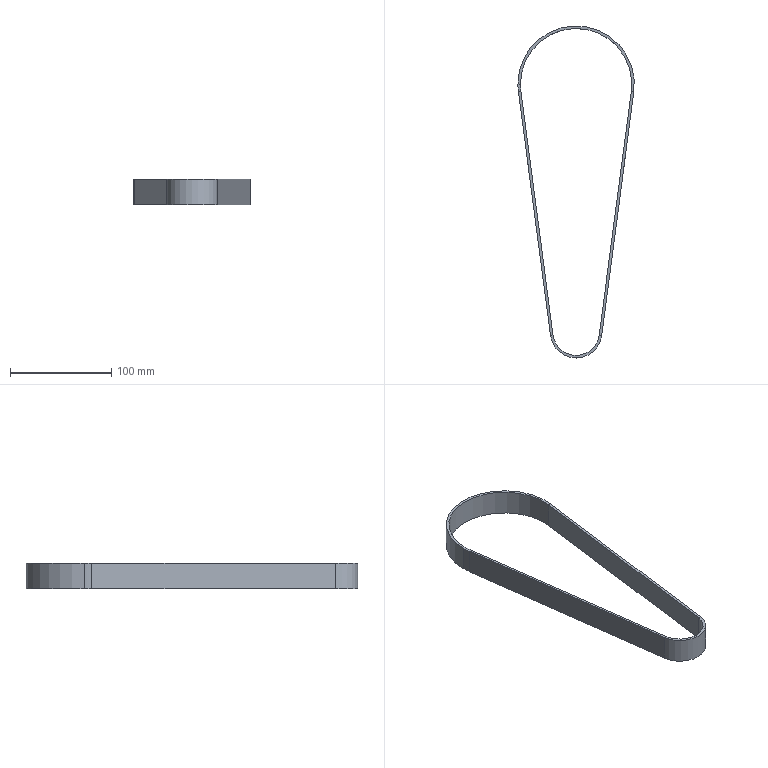Part | 1 solid | 20 faces | box 115 x 328 x 25 mm | volume 46693 mm3 | plane 14 | cylinder 6 | commonest cylinder face diameters 110 x2 115 x2 46 x1 51 x1
STEP:
#1=CARTESIAN_POINT('',(-54.529,-7.184,-12.5));
#2=VERTEX_POINT('',#1);
#3=CARTESIAN_POINT('',(-55.,0.,-12.5));
#4=VERTEX_POINT('',#3);
#5=CARTESIAN_POINT('',(0.,0.,-12.5));
#6=DIRECTION('',(0.,0.,-1.));
#7=DIRECTION('',(-0.9914,-0.1306,0.));
#8=AXIS2_PLACEMENT_3D('',#5,#6,#7);
#9=CIRCLE('',#8,55.);
#10=EDGE_CURVE('',#2,#4,#9,.T.);
#11=ORIENTED_EDGE('',*,*,#10,.F.);
#12=CARTESIAN_POINT('',(-57.007,-7.51,-12.5));
#13=VERTEX_POINT('',#12);
#14=CARTESIAN_POINT('',(-57.007,-7.51,-12.5));
#15=DIRECTION('',(-0.9914,-0.1306,0.));
#16=VECTOR('',#15,1000.);
#17=LINE('',#14,#16);
#18=EDGE_CURVE('',#2,#13,#17,.T.);
#19=ORIENTED_EDGE('',*,*,#18,.T.);
#20=CARTESIAN_POINT('',(-57.5,0.,-12.5));
#21=VERTEX_POINT('',#20);
#22=CARTESIAN_POINT('',(0.,0.,-12.5));
#23=DIRECTION('',(0.,0.,-1.));
#24=DIRECTION('',(-0.9914,-0.1306,0.));
#25=AXIS2_PLACEMENT_3D('',#22,#23,#24);
#26=CIRCLE('',#25,57.5);
#27=EDGE_CURVE('',#13,#21,#26,.T.);
#28=ORIENTED_EDGE('',*,*,#27,.T.);
#29=CARTESIAN_POINT('',(-57.5,0.,-12.5));
#30=DIRECTION('',(-1.,0.,0.));
#31=VECTOR('',#30,1000.);
#32=LINE('',#29,#31);
#33=EDGE_CURVE('',#4,#21,#32,.T.);
#34=ORIENTED_EDGE('',*,*,#33,.F.);
#35=EDGE_LOOP('',(#11,#19,#28,#34));
#36=FACE_OUTER_BOUND('',#35,.T.);
#37=CARTESIAN_POINT('',(-57.007,-7.51,-12.5));
#38=DIRECTION('',(0.,0.,-1.));
#39=DIRECTION('',(-1.,0.,0.));
#40=AXIS2_PLACEMENT_3D('',#37,#38,#39);
#41=PLANE('',#40);
#42=ADVANCED_FACE('',(#36),#41,.T.);
#43=CARTESIAN_POINT('',(-54.529,-7.184,12.5));
#44=VERTEX_POINT('',#43);
#45=CARTESIAN_POINT('',(-55.,0.,12.5));
#46=VERTEX_POINT('',#45);
#47=CARTESIAN_POINT('',(0.,0.,12.5));
#48=DIRECTION('',(0.,0.,-1.));
#49=DIRECTION('',(-0.9914,-0.1306,0.));
#50=AXIS2_PLACEMENT_3D('',#47,#48,#49);
#51=CIRCLE('',#50,55.);
#52=EDGE_CURVE('',#44,#46,#51,.T.);
#53=ORIENTED_EDGE('',*,*,#52,.F.);
#54=CARTESIAN_POINT('',(-54.529,-7.184,-12.5));
#55=DIRECTION('',(0.,0.,-1.));
#56=VECTOR('',#55,1000.);
#57=LINE('',#54,#56);
#58=EDGE_CURVE('',#44,#2,#57,.T.);
#59=ORIENTED_EDGE('',*,*,#58,.T.);
#60=ORIENTED_EDGE('',*,*,#10,.T.);
#61=CARTESIAN_POINT('',(-55.,0.,-12.5));
#62=DIRECTION('',(0.,0.,-1.));
#63=VECTOR('',#62,1000.);
#64=LINE('',#61,#63);
#65=EDGE_CURVE('',#46,#4,#64,.T.);
#66=ORIENTED_EDGE('',*,*,#65,.F.);
#67=EDGE_LOOP('',(#53,#59,#60,#66));
#68=FACE_OUTER_BOUND('',#67,.T.);
#69=CARTESIAN_POINT('',(0.,0.,0.));
#70=DIRECTION('',(0.,0.,-1.));
#71=DIRECTION('',(-1.,0.,0.));
#72=AXIS2_PLACEMENT_3D('',#69,#70,#71);
#73=CYLINDRICAL_SURFACE('',#72,55.);
#74=ADVANCED_FACE('',(#68),#73,.F.);
#75=CARTESIAN_POINT('',(-57.007,-7.51,12.5));
#76=VERTEX_POINT('',#75);
#77=CARTESIAN_POINT('',(-57.5,0.,12.5));
#78=VERTEX_POINT('',#77);
#79=CARTESIAN_POINT('',(0.,0.,12.5));
#80=DIRECTION('',(0.,0.,-1.));
#81=DIRECTION('',(-0.9914,-0.1306,0.));
#82=AXIS2_PLACEMENT_3D('',#79,#80,#81);
#83=CIRCLE('',#82,57.5);
#84=EDGE_CURVE('',#76,#78,#83,.T.);
#85=ORIENTED_EDGE('',*,*,#84,.F.);
#86=CARTESIAN_POINT('',(-57.007,-7.51,12.5));
#87=DIRECTION('',(0.9914,0.1306,0.));
#88=VECTOR('',#87,1000.);
#89=LINE('',#86,#88);
#90=EDGE_CURVE('',#76,#44,#89,.T.);
#91=ORIENTED_EDGE('',*,*,#90,.T.);
#92=ORIENTED_EDGE('',*,*,#52,.T.);
#93=CARTESIAN_POINT('',(-57.5,0.,12.5));
#94=DIRECTION('',(1.,0.,0.));
#95=VECTOR('',#94,1000.);
#96=LINE('',#93,#95);
#97=EDGE_CURVE('',#78,#46,#96,.T.);
#98=ORIENTED_EDGE('',*,*,#97,.F.);
#99=EDGE_LOOP('',(#85,#91,#92,#98));
#100=FACE_OUTER_BOUND('',#99,.T.);
#101=CARTESIAN_POINT('',(-57.007,-7.51,12.5));
#102=DIRECTION('',(0.,0.,1.));
#103=DIRECTION('',(1.,0.,0.));
#104=AXIS2_PLACEMENT_3D('',#101,#102,#103);
#105=PLANE('',#104);
#106=ADVANCED_FACE('',(#100),#105,.T.);
#107=ORIENTED_EDGE('',*,*,#18,.F.);
#108=CARTESIAN_POINT('',(-22.803,-248.004,-12.5));
#109=VERTEX_POINT('',#108);
#110=CARTESIAN_POINT('',(-22.803,-248.004,-12.5));
#111=DIRECTION('',(-0.1306,0.9914,0.));
#112=VECTOR('',#111,1000.);
#113=LINE('',#110,#112);
#114=EDGE_CURVE('',#109,#2,#113,.T.);
#115=ORIENTED_EDGE('',*,*,#114,.F.);
#116=CARTESIAN_POINT('',(-25.282,-248.331,-12.5));
#117=VERTEX_POINT('',#116);
#118=CARTESIAN_POINT('',(-25.282,-248.331,-12.5));
#119=DIRECTION('',(-0.9914,-0.1306,0.));
#120=VECTOR('',#119,1000.);
#121=LINE('',#118,#120);
#122=EDGE_CURVE('',#109,#117,#121,.T.);
#123=ORIENTED_EDGE('',*,*,#122,.T.);
#124=CARTESIAN_POINT('',(-25.282,-248.331,-12.5));
#125=DIRECTION('',(-0.1306,0.9914,0.));
#126=VECTOR('',#125,1000.);
#127=LINE('',#124,#126);
#128=EDGE_CURVE('',#117,#13,#127,.T.);
#129=ORIENTED_EDGE('',*,*,#128,.T.);
#130=EDGE_LOOP('',(#107,#115,#123,#129));
#131=FACE_OUTER_BOUND('',#130,.T.);
#132=CARTESIAN_POINT('',(-25.282,-248.331,-12.5));
#133=DIRECTION('',(0.,0.,-1.));
#134=DIRECTION('',(-1.,0.,0.));
#135=AXIS2_PLACEMENT_3D('',#132,#133,#134);
#136=PLANE('',#135);
#137=ADVANCED_FACE('',(#131),#136,.T.);
#138=ORIENTED_EDGE('',*,*,#114,.T.);
#139=ORIENTED_EDGE('',*,*,#58,.F.);
#140=CARTESIAN_POINT('',(-22.803,-248.004,12.5));
#141=VERTEX_POINT('',#140);
#142=CARTESIAN_POINT('',(-22.803,-248.004,12.5));
#143=DIRECTION('',(-0.1306,0.9914,0.));
#144=VECTOR('',#143,1000.);
#145=LINE('',#142,#144);
#146=EDGE_CURVE('',#141,#44,#145,.T.);
#147=ORIENTED_EDGE('',*,*,#146,.F.);
#148=CARTESIAN_POINT('',(-22.803,-248.004,-12.5));
#149=DIRECTION('',(0.,0.,-1.));
#150=VECTOR('',#149,1000.);
#151=LINE('',#148,#150);
#152=EDGE_CURVE('',#141,#109,#151,.T.);
#153=ORIENTED_EDGE('',*,*,#152,.T.);
#154=EDGE_LOOP('',(#138,#139,#147,#153));
#155=FACE_OUTER_BOUND('',#154,.T.);
#156=CARTESIAN_POINT('',(-22.803,-248.004,-12.5));
#157=DIRECTION('',(0.9914,0.1306,0.));
#158=DIRECTION('',(-0.1306,0.9914,0.));
#159=AXIS2_PLACEMENT_3D('',#156,#157,#158);
#160=PLANE('',#159);
#161=ADVANCED_FACE('',(#155),#160,.T.);
#162=ORIENTED_EDGE('',*,*,#146,.T.);
#163=ORIENTED_EDGE('',*,*,#90,.F.);
#164=CARTESIAN_POINT('',(-25.282,-248.331,12.5));
#165=VERTEX_POINT('',#164);
#166=CARTESIAN_POINT('',(-25.282,-248.331,12.5));
#167=DIRECTION('',(-0.1306,0.9914,0.));
#168=VECTOR('',#167,1000.);
#169=LINE('',#166,#168);
#170=EDGE_CURVE('',#165,#76,#169,.T.);
#171=ORIENTED_EDGE('',*,*,#170,.F.);
#172=CARTESIAN_POINT('',(-25.282,-248.331,12.5));
#173=DIRECTION('',(0.9914,0.1306,0.));
#174=VECTOR('',#173,1000.);
#175=LINE('',#172,#174);
#176=EDGE_CURVE('',#165,#141,#175,.T.);
#177=ORIENTED_EDGE('',*,*,#176,.T.);
#178=EDGE_LOOP('',(#162,#163,#171,#177));
#179=FACE_OUTER_BOUND('',#178,.T.);
#180=CARTESIAN_POINT('',(-25.282,-248.331,12.5));
#181=DIRECTION('',(0.,0.,1.));
#182=DIRECTION('',(1.,0.,0.));
#183=AXIS2_PLACEMENT_3D('',#180,#181,#182);
#184=PLANE('',#183);
#185=ADVANCED_FACE('',(#179),#184,.T.);
#186=ORIENTED_EDGE('',*,*,#170,.T.);
#187=CARTESIAN_POINT('',(-57.007,-7.51,-12.5));
#188=DIRECTION('',(0.,0.,1.));
#189=VECTOR('',#188,1000.);
#190=LINE('',#187,#189);
#191=EDGE_CURVE('',#13,#76,#190,.T.);
#192=ORIENTED_EDGE('',*,*,#191,.F.);
#193=ORIENTED_EDGE('',*,*,#128,.F.);
#194=CARTESIAN_POINT('',(-25.282,-248.331,-12.5));
#195=DIRECTION('',(0.,0.,1.));
#196=VECTOR('',#195,1000.);
#197=LINE('',#194,#196);
#198=EDGE_CURVE('',#117,#165,#197,.T.);
#199=ORIENTED_EDGE('',*,*,#198,.T.);
#200=EDGE_LOOP('',(#186,#192,#193,#199));
#201=FACE_OUTER_BOUND('',#200,.T.);
#202=CARTESIAN_POINT('',(-25.282,-248.331,-12.5));
#203=DIRECTION('',(-0.9914,-0.1306,0.));
#204=DIRECTION('',(0.1306,-0.9914,0.));
#205=AXIS2_PLACEMENT_3D('',#202,#203,#204);
#206=PLANE('',#205);
#207=ADVANCED_FACE('',(#201),#206,.T.);
#208=ORIENTED_EDGE('',*,*,#122,.F.);
#209=CARTESIAN_POINT('',(22.803,-248.004,-12.5));
#210=VERTEX_POINT('',#209);
#211=CARTESIAN_POINT('',(0.,-245.,-12.5));
#212=DIRECTION('',(0.,0.,-1.));
#213=DIRECTION('',(0.9914,-0.1306,0.));
#214=AXIS2_PLACEMENT_3D('',#211,#212,#213);
#215=CIRCLE('',#214,23.);
#216=EDGE_CURVE('',#210,#109,#215,.T.);
#217=ORIENTED_EDGE('',*,*,#216,.F.);
#218=CARTESIAN_POINT('',(25.282,-248.331,-12.5));
#219=VERTEX_POINT('',#218);
#220=CARTESIAN_POINT('',(25.282,-248.331,-12.5));
#221=DIRECTION('',(0.9914,-0.1306,0.));
#222=VECTOR('',#221,1000.);
#223=LINE('',#220,#222);
#224=EDGE_CURVE('',#210,#219,#223,.T.);
#225=ORIENTED_EDGE('',*,*,#224,.T.);
#226=CARTESIAN_POINT('',(0.,-245.,-12.5));
#227=DIRECTION('',(0.,0.,-1.));
#228=DIRECTION('',(0.9914,-0.1306,0.));
#229=AXIS2_PLACEMENT_3D('',#226,#227,#228);
#230=CIRCLE('',#229,25.5);
#231=EDGE_CURVE('',#219,#117,#230,.T.);
#232=ORIENTED_EDGE('',*,*,#231,.T.);
#233=EDGE_LOOP('',(#208,#217,#225,#232));
#234=FACE_OUTER_BOUND('',#233,.T.);
#235=CARTESIAN_POINT('',(25.282,-248.331,-12.5));
#236=DIRECTION('',(0.,0.,-1.));
#237=DIRECTION('',(-1.,0.,0.));
#238=AXIS2_PLACEMENT_3D('',#235,#236,#237);
#239=PLANE('',#238);
#240=ADVANCED_FACE('',(#234),#239,.T.);
#241=ORIENTED_EDGE('',*,*,#216,.T.);
#242=ORIENTED_EDGE('',*,*,#152,.F.);
#243=CARTESIAN_POINT('',(22.803,-248.004,12.5));
#244=VERTEX_POINT('',#243);
#245=CARTESIAN_POINT('',(0.,-245.,12.5));
#246=DIRECTION('',(0.,0.,-1.));
#247=DIRECTION('',(0.9914,-0.1306,0.));
#248=AXIS2_PLACEMENT_3D('',#245,#246,#247);
#249=CIRCLE('',#248,23.);
#250=EDGE_CURVE('',#244,#141,#249,.T.);
#251=ORIENTED_EDGE('',*,*,#250,.F.);
#252=CARTESIAN_POINT('',(22.803,-248.004,-12.5));
#253=DIRECTION('',(0.,0.,-1.));
#254=VECTOR('',#253,1000.);
#255=LINE('',#252,#254);
#256=EDGE_CURVE('',#244,#210,#255,.T.);
#257=ORIENTED_EDGE('',*,*,#256,.T.);
#258=EDGE_LOOP('',(#241,#242,#251,#257));
#259=FACE_OUTER_BOUND('',#258,.T.);
#260=CARTESIAN_POINT('',(0.,-245.,0.));
#261=DIRECTION('',(0.,0.,-1.));
#262=DIRECTION('',(-1.,0.,0.));
#263=AXIS2_PLACEMENT_3D('',#260,#261,#262);
#264=CYLINDRICAL_SURFACE('',#263,23.);
#265=ADVANCED_FACE('',(#259),#264,.F.);
#266=ORIENTED_EDGE('',*,*,#250,.T.);
#267=ORIENTED_EDGE('',*,*,#176,.F.);
#268=CARTESIAN_POINT('',(25.282,-248.331,12.5));
#269=VERTEX_POINT('',#268);
#270=CARTESIAN_POINT('',(0.,-245.,12.5));
#271=DIRECTION('',(0.,0.,-1.));
#272=DIRECTION('',(0.9914,-0.1306,0.));
#273=AXIS2_PLACEMENT_3D('',#270,#271,#272);
#274=CIRCLE('',#273,25.5);
#275=EDGE_CURVE('',#269,#165,#274,.T.);
#276=ORIENTED_EDGE('',*,*,#275,.F.);
#277=CARTESIAN_POINT('',(25.282,-248.331,12.5));
#278=DIRECTION('',(-0.9914,0.1306,0.));
#279=VECTOR('',#278,1000.);
#280=LINE('',#277,#279);
#281=EDGE_CURVE('',#269,#244,#280,.T.);
#282=ORIENTED_EDGE('',*,*,#281,.T.);
#283=EDGE_LOOP('',(#266,#267,#276,#282));
#284=FACE_OUTER_BOUND('',#283,.T.);
#285=CARTESIAN_POINT('',(25.282,-248.331,12.5));
#286=DIRECTION('',(0.,0.,1.));
#287=DIRECTION('',(1.,0.,0.));
#288=AXIS2_PLACEMENT_3D('',#285,#286,#287);
#289=PLANE('',#288);
#290=ADVANCED_FACE('',(#284),#289,.T.);
#291=ORIENTED_EDGE('',*,*,#275,.T.);
#292=ORIENTED_EDGE('',*,*,#198,.F.);
#293=ORIENTED_EDGE('',*,*,#231,.F.);
#294=CARTESIAN_POINT('',(25.282,-248.331,-12.5));
#295=DIRECTION('',(0.,0.,1.));
#296=VECTOR('',#295,1000.);
#297=LINE('',#294,#296);
#298=EDGE_CURVE('',#219,#269,#297,.T.);
#299=ORIENTED_EDGE('',*,*,#298,.T.);
#300=EDGE_LOOP('',(#291,#292,#293,#299));
#301=FACE_OUTER_BOUND('',#300,.T.);
#302=CARTESIAN_POINT('',(0.,-245.,0.));
#303=DIRECTION('',(0.,0.,-1.));
#304=DIRECTION('',(-1.,0.,0.));
#305=AXIS2_PLACEMENT_3D('',#302,#303,#304);
#306=CYLINDRICAL_SURFACE('',#305,25.5);
#307=ADVANCED_FACE('',(#301),#306,.T.);
#308=ORIENTED_EDGE('',*,*,#224,.F.);
#309=CARTESIAN_POINT('',(54.529,-7.184,-12.5));
#310=VERTEX_POINT('',#309);
#311=CARTESIAN_POINT('',(54.529,-7.184,-12.5));
#312=DIRECTION('',(-0.1306,-0.9914,0.));
#313=VECTOR('',#312,1000.);
#314=LINE('',#311,#313);
#315=EDGE_CURVE('',#310,#210,#314,.T.);
#316=ORIENTED_EDGE('',*,*,#315,.F.);
#317=CARTESIAN_POINT('',(57.007,-7.51,-12.5));
#318=VERTEX_POINT('',#317);
#319=CARTESIAN_POINT('',(57.007,-7.51,-12.5));
#320=DIRECTION('',(0.9914,-0.1306,0.));
#321=VECTOR('',#320,1000.);
#322=LINE('',#319,#321);
#323=EDGE_CURVE('',#310,#318,#322,.T.);
#324=ORIENTED_EDGE('',*,*,#323,.T.);
#325=CARTESIAN_POINT('',(57.007,-7.51,-12.5));
#326=DIRECTION('',(-0.1306,-0.9914,0.));
#327=VECTOR('',#326,1000.);
#328=LINE('',#325,#327);
#329=EDGE_CURVE('',#318,#219,#328,.T.);
#330=ORIENTED_EDGE('',*,*,#329,.T.);
#331=EDGE_LOOP('',(#308,#316,#324,#330));
#332=FACE_OUTER_BOUND('',#331,.T.);
#333=CARTESIAN_POINT('',(57.007,-7.51,-12.5));
#334=DIRECTION('',(0.,0.,-1.));
#335=DIRECTION('',(-1.,0.,0.));
#336=AXIS2_PLACEMENT_3D('',#333,#334,#335);
#337=PLANE('',#336);
#338=ADVANCED_FACE('',(#332),#337,.T.);
#339=ORIENTED_EDGE('',*,*,#315,.T.);
#340=ORIENTED_EDGE('',*,*,#256,.F.);
#341=CARTESIAN_POINT('',(54.529,-7.184,12.5));
#342=VERTEX_POINT('',#341);
#343=CARTESIAN_POINT('',(54.529,-7.184,12.5));
#344=DIRECTION('',(-0.1306,-0.9914,0.));
#345=VECTOR('',#344,1000.);
#346=LINE('',#343,#345);
#347=EDGE_CURVE('',#342,#244,#346,.T.);
#348=ORIENTED_EDGE('',*,*,#347,.F.);
#349=CARTESIAN_POINT('',(54.529,-7.184,-12.5));
#350=DIRECTION('',(0.,0.,-1.));
#351=VECTOR('',#350,1000.);
#352=LINE('',#349,#351);
#353=EDGE_CURVE('',#342,#310,#352,.T.);
#354=ORIENTED_EDGE('',*,*,#353,.T.);
#355=EDGE_LOOP('',(#339,#340,#348,#354));
#356=FACE_OUTER_BOUND('',#355,.T.);
#357=CARTESIAN_POINT('',(54.529,-7.184,-12.5));
#358=DIRECTION('',(-0.9914,0.1306,0.));
#359=DIRECTION('',(-0.1306,-0.9914,0.));
#360=AXIS2_PLACEMENT_3D('',#357,#358,#359);
#361=PLANE('',#360);
#362=ADVANCED_FACE('',(#356),#361,.T.);
#363=ORIENTED_EDGE('',*,*,#347,.T.);
#364=ORIENTED_EDGE('',*,*,#281,.F.);
#365=CARTESIAN_POINT('',(57.007,-7.51,12.5));
#366=VERTEX_POINT('',#365);
#367=CARTESIAN_POINT('',(57.007,-7.51,12.5));
#368=DIRECTION('',(-0.1306,-0.9914,0.));
#369=VECTOR('',#368,1000.);
#370=LINE('',#367,#369);
#371=EDGE_CURVE('',#366,#269,#370,.T.);
#372=ORIENTED_EDGE('',*,*,#371,.F.);
#373=CARTESIAN_POINT('',(57.007,-7.51,12.5));
#374=DIRECTION('',(-0.9914,0.1306,0.));
#375=VECTOR('',#374,1000.);
#376=LINE('',#373,#375);
#377=EDGE_CURVE('',#366,#342,#376,.T.);
#378=ORIENTED_EDGE('',*,*,#377,.T.);
#379=EDGE_LOOP('',(#363,#364,#372,#378));
#380=FACE_OUTER_BOUND('',#379,.T.);
#381=CARTESIAN_POINT('',(57.007,-7.51,12.5));
#382=DIRECTION('',(0.,0.,1.));
#383=DIRECTION('',(1.,0.,0.));
#384=AXIS2_PLACEMENT_3D('',#381,#382,#383);
#385=PLANE('',#384);
#386=ADVANCED_FACE('',(#380),#385,.T.);
#387=ORIENTED_EDGE('',*,*,#371,.T.);
#388=ORIENTED_EDGE('',*,*,#298,.F.);
#389=ORIENTED_EDGE('',*,*,#329,.F.);
#390=CARTESIAN_POINT('',(57.007,-7.51,-12.5));
#391=DIRECTION('',(0.,0.,1.));
#392=VECTOR('',#391,1000.);
#393=LINE('',#390,#392);
#394=EDGE_CURVE('',#318,#366,#393,.T.);
#395=ORIENTED_EDGE('',*,*,#394,.T.);
#396=EDGE_LOOP('',(#387,#388,#389,#395));
#397=FACE_OUTER_BOUND('',#396,.T.);
#398=CARTESIAN_POINT('',(57.007,-7.51,-12.5));
#399=DIRECTION('',(0.9914,-0.1306,0.));
#400=DIRECTION('',(0.1306,0.9914,0.));
#401=AXIS2_PLACEMENT_3D('',#398,#399,#400);
#402=PLANE('',#401);
#403=ADVANCED_FACE('',(#397),#402,.T.);
#404=ORIENTED_EDGE('',*,*,#323,.F.);
#405=CARTESIAN_POINT('',(0.,0.,-12.5));
#406=DIRECTION('',(0.,0.,-1.));
#407=DIRECTION('',(-1.,0.,0.));
#408=AXIS2_PLACEMENT_3D('',#405,#406,#407);
#409=CIRCLE('',#408,55.);
#410=EDGE_CURVE('',#4,#310,#409,.T.);
#411=ORIENTED_EDGE('',*,*,#410,.F.);
#412=ORIENTED_EDGE('',*,*,#33,.T.);
#413=CARTESIAN_POINT('',(0.,0.,-12.5));
#414=DIRECTION('',(0.,0.,-1.));
#415=DIRECTION('',(-1.,0.,0.));
#416=AXIS2_PLACEMENT_3D('',#413,#414,#415);
#417=CIRCLE('',#416,57.5);
#418=EDGE_CURVE('',#21,#318,#417,.T.);
#419=ORIENTED_EDGE('',*,*,#418,.T.);
#420=EDGE_LOOP('',(#404,#411,#412,#419));
#421=FACE_OUTER_BOUND('',#420,.T.);
#422=CARTESIAN_POINT('',(-57.5,0.,-12.5));
#423=DIRECTION('',(0.,0.,-1.));
#424=DIRECTION('',(-1.,0.,0.));
#425=AXIS2_PLACEMENT_3D('',#422,#423,#424);
#426=PLANE('',#425);
#427=ADVANCED_FACE('',(#421),#426,.T.);
#428=ORIENTED_EDGE('',*,*,#410,.T.);
#429=ORIENTED_EDGE('',*,*,#353,.F.);
#430=CARTESIAN_POINT('',(0.,0.,12.5));
#431=DIRECTION('',(0.,0.,-1.));
#432=DIRECTION('',(-1.,0.,0.));
#433=AXIS2_PLACEMENT_3D('',#430,#431,#432);
#434=CIRCLE('',#433,55.);
#435=EDGE_CURVE('',#46,#342,#434,.T.);
#436=ORIENTED_EDGE('',*,*,#435,.F.);
#437=ORIENTED_EDGE('',*,*,#65,.T.);
#438=EDGE_LOOP('',(#428,#429,#436,#437));
#439=FACE_OUTER_BOUND('',#438,.T.);
#440=CARTESIAN_POINT('',(0.,0.,0.));
#441=DIRECTION('',(0.,0.,-1.));
#442=DIRECTION('',(-1.,0.,0.));
#443=AXIS2_PLACEMENT_3D('',#440,#441,#442);
#444=CYLINDRICAL_SURFACE('',#443,55.);
#445=ADVANCED_FACE('',(#439),#444,.F.);
#446=ORIENTED_EDGE('',*,*,#435,.T.);
#447=ORIENTED_EDGE('',*,*,#377,.F.);
#448=CARTESIAN_POINT('',(0.,0.,12.5));
#449=DIRECTION('',(0.,0.,-1.));
#450=DIRECTION('',(-1.,0.,0.));
#451=AXIS2_PLACEMENT_3D('',#448,#449,#450);
#452=CIRCLE('',#451,57.5);
#453=EDGE_CURVE('',#78,#366,#452,.T.);
#454=ORIENTED_EDGE('',*,*,#453,.F.);
#455=ORIENTED_EDGE('',*,*,#97,.T.);
#456=EDGE_LOOP('',(#446,#447,#454,#455));
#457=FACE_OUTER_BOUND('',#456,.T.);
#458=CARTESIAN_POINT('',(-57.5,0.,12.5));
#459=DIRECTION('',(0.,0.,1.));
#460=DIRECTION('',(1.,0.,0.));
#461=AXIS2_PLACEMENT_3D('',#458,#459,#460);
#462=PLANE('',#461);
#463=ADVANCED_FACE('',(#457),#462,.T.);
#464=ORIENTED_EDGE('',*,*,#453,.T.);
#465=ORIENTED_EDGE('',*,*,#394,.F.);
#466=ORIENTED_EDGE('',*,*,#418,.F.);
#467=CARTESIAN_POINT('',(-57.5,0.,-12.5));
#468=DIRECTION('',(0.,0.,1.));
#469=VECTOR('',#468,1000.);
#470=LINE('',#467,#469);
#471=EDGE_CURVE('',#21,#78,#470,.T.);
#472=ORIENTED_EDGE('',*,*,#471,.T.);
#473=EDGE_LOOP('',(#464,#465,#466,#472));
#474=FACE_OUTER_BOUND('',#473,.T.);
#475=CARTESIAN_POINT('',(0.,0.,0.));
#476=DIRECTION('',(0.,0.,-1.));
#477=DIRECTION('',(-1.,0.,0.));
#478=AXIS2_PLACEMENT_3D('',#475,#476,#477);
#479=CYLINDRICAL_SURFACE('',#478,57.5);
#480=ADVANCED_FACE('',(#474),#479,.T.);
#481=ORIENTED_EDGE('',*,*,#191,.T.);
#482=ORIENTED_EDGE('',*,*,#84,.T.);
#483=ORIENTED_EDGE('',*,*,#471,.F.);
#484=ORIENTED_EDGE('',*,*,#27,.F.);
#485=EDGE_LOOP('',(#481,#482,#483,#484));
#486=FACE_OUTER_BOUND('',#485,.T.);
#487=CARTESIAN_POINT('',(0.,0.,0.));
#488=DIRECTION('',(0.,0.,-1.));
#489=DIRECTION('',(-1.,0.,0.));
#490=AXIS2_PLACEMENT_3D('',#487,#488,#489);
#491=CYLINDRICAL_SURFACE('',#490,57.5);
#492=ADVANCED_FACE('',(#486),#491,.T.);
#493=CLOSED_SHELL('',(#42,#74,#106,#137,#161,#185,#207,#240,#265,#290,#307,#338,#362,#386,#403,#427,#445,#463,#480,#492));
#494=MANIFOLD_SOLID_BREP('',#493);
#495=CARTESIAN_POINT('',(0.,0.,0.));
#496=DIRECTION('',(0.,0.,1.));
#497=DIRECTION('',(1.,0.,0.));
#498=AXIS2_PLACEMENT_3D('',#495,#496,#497);
#499=(LENGTH_UNIT()NAMED_UNIT(*)SI_UNIT(.MILLI.,.METRE.));
#500=UNCERTAINTY_MEASURE_WITH_UNIT(LENGTH_MEASURE(0.00001),#499,'','');
#501=(NAMED_UNIT(*)PLANE_ANGLE_UNIT()SI_UNIT($,.RADIAN.));
#502=(NAMED_UNIT(*)SI_UNIT($,.STERADIAN.)SOLID_ANGLE_UNIT());
#503=(GEOMETRIC_REPRESENTATION_CONTEXT(3)GLOBAL_UNCERTAINTY_ASSIGNED_CONTEXT((#500))GLOBAL_UNIT_ASSIGNED_CONTEXT((#499,#501,#502))REPRESENTATION_CONTEXT('',''));
#504=ADVANCED_BREP_SHAPE_REPRESENTATION('',(#494,#498),#503);